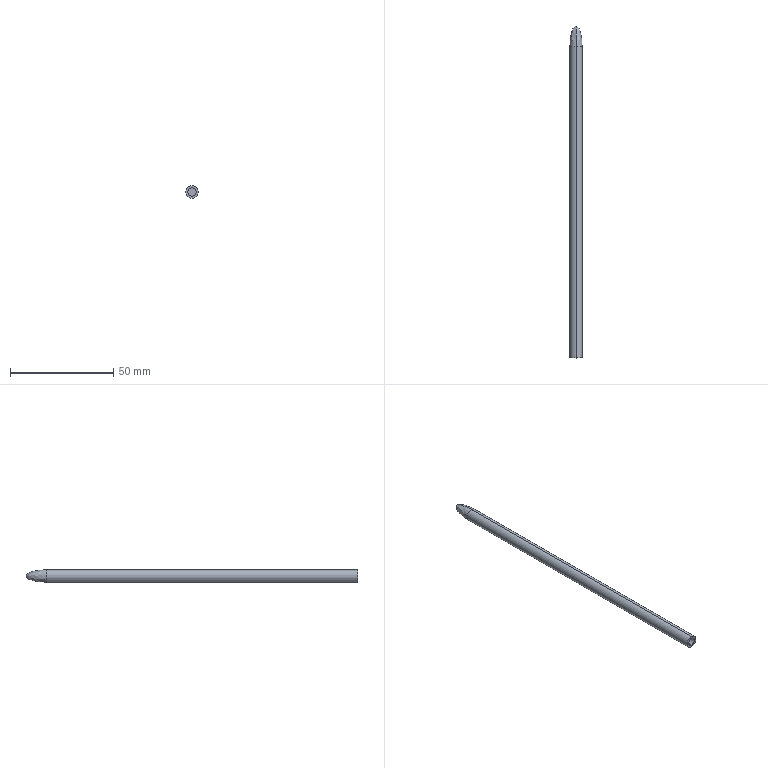Part | SolidWorks | features BaseBody 1 | 1 solid | 8 faces | box 6 x 161 x 6 mm | volume 2573 mm3 | cylinder 4 | plane 2 | spline 2 | commonest cylinder face diameters 4 x2 6 x2
STEP:
#1=CARTESIAN_POINT('',(0.,83.134,-3.));
#2=VERTEX_POINT('',#1);
#3=CARTESIAN_POINT('',(0.,83.134,3.));
#4=VERTEX_POINT('',#3);
#5=CARTESIAN_POINT('',(0.,83.134,0.));
#6=DIRECTION('',(0.,-1.,0.));
#7=DIRECTION('',(0.,0.,-1.));
#8=AXIS2_PLACEMENT_3D('',#5,#6,#7);
#9=CIRCLE('',#8,3.);
#10=EDGE_CURVE('',#2,#4,#9,.T.);
#11=ORIENTED_EDGE('',*,*,#10,.T.);
#12=CARTESIAN_POINT('',(0.,-67.866,3.));
#13=VERTEX_POINT('',#12);
#14=CARTESIAN_POINT('',(0.,0.,3.));
#15=DIRECTION('',(0.,-1.,0.));
#16=VECTOR('',#15,1000.);
#17=LINE('',#14,#16);
#18=EDGE_CURVE('',#4,#13,#17,.T.);
#19=ORIENTED_EDGE('',*,*,#18,.T.);
#20=CARTESIAN_POINT('',(0.,-67.866,-3.));
#21=VERTEX_POINT('',#20);
#22=CARTESIAN_POINT('',(0.,-67.866,0.));
#23=DIRECTION('',(0.,1.,0.));
#24=DIRECTION('',(0.,0.,-1.));
#25=AXIS2_PLACEMENT_3D('',#22,#23,#24);
#26=CIRCLE('',#25,3.);
#27=EDGE_CURVE('',#13,#21,#26,.T.);
#28=ORIENTED_EDGE('',*,*,#27,.T.);
#29=CARTESIAN_POINT('',(0.,0.,-3.));
#30=DIRECTION('',(0.,-1.,0.));
#31=VECTOR('',#30,1000.);
#32=LINE('',#29,#31);
#33=EDGE_CURVE('',#2,#21,#32,.T.);
#34=ORIENTED_EDGE('',*,*,#33,.F.);
#35=EDGE_LOOP('',(#11,#19,#28,#34));
#36=FACE_OUTER_BOUND('',#35,.T.);
#37=CARTESIAN_POINT('',(0.,0.,0.));
#38=DIRECTION('',(0.,-1.,0.));
#39=DIRECTION('',(0.,0.,-1.));
#40=AXIS2_PLACEMENT_3D('',#37,#38,#39);
#41=CYLINDRICAL_SURFACE('',#40,3.);
#42=ADVANCED_FACE('',(#36),#41,.T.);
#43=CARTESIAN_POINT('',(0.,82.134,2.));
#44=VERTEX_POINT('',#43);
#45=CARTESIAN_POINT('',(0.,82.134,-2.));
#46=VERTEX_POINT('',#45);
#47=CARTESIAN_POINT('',(0.,82.134,0.));
#48=DIRECTION('',(0.,-1.,0.));
#49=DIRECTION('',(0.,0.,-1.));
#50=AXIS2_PLACEMENT_3D('',#47,#48,#49);
#51=CIRCLE('',#50,2.);
#52=EDGE_CURVE('',#44,#46,#51,.T.);
#53=ORIENTED_EDGE('',*,*,#52,.F.);
#54=CARTESIAN_POINT('',(0.,-67.866,2.));
#55=VERTEX_POINT('',#54);
#56=CARTESIAN_POINT('',(0.,0.,2.));
#57=DIRECTION('',(0.,-1.,0.));
#58=VECTOR('',#57,1000.);
#59=LINE('',#56,#58);
#60=EDGE_CURVE('',#44,#55,#59,.T.);
#61=ORIENTED_EDGE('',*,*,#60,.T.);
#62=CARTESIAN_POINT('',(0.,-67.866,-2.));
#63=VERTEX_POINT('',#62);
#64=CARTESIAN_POINT('',(0.,-67.866,0.));
#65=DIRECTION('',(0.,-1.,0.));
#66=DIRECTION('',(0.,0.,-1.));
#67=AXIS2_PLACEMENT_3D('',#64,#65,#66);
#68=CIRCLE('',#67,2.);
#69=EDGE_CURVE('',#55,#63,#68,.T.);
#70=ORIENTED_EDGE('',*,*,#69,.T.);
#71=CARTESIAN_POINT('',(0.,0.,-2.));
#72=DIRECTION('',(0.,-1.,0.));
#73=VECTOR('',#72,1000.);
#74=LINE('',#71,#73);
#75=EDGE_CURVE('',#46,#63,#74,.T.);
#76=ORIENTED_EDGE('',*,*,#75,.F.);
#77=EDGE_LOOP('',(#53,#61,#70,#76));
#78=FACE_OUTER_BOUND('',#77,.T.);
#79=CARTESIAN_POINT('',(0.,0.,0.));
#80=DIRECTION('',(0.,-1.,0.));
#81=DIRECTION('',(0.,0.,-1.));
#82=AXIS2_PLACEMENT_3D('',#79,#80,#81);
#83=CYLINDRICAL_SURFACE('',#82,2.);
#84=ADVANCED_FACE('',(#78),#83,.F.);
#85=ORIENTED_EDGE('',*,*,#18,.F.);
#86=CARTESIAN_POINT('',(0.,83.134,0.));
#87=DIRECTION('',(0.,-1.,0.));
#88=DIRECTION('',(0.,0.,-1.));
#89=AXIS2_PLACEMENT_3D('',#86,#87,#88);
#90=CIRCLE('',#89,3.);
#91=EDGE_CURVE('',#4,#2,#90,.T.);
#92=ORIENTED_EDGE('',*,*,#91,.T.);
#93=ORIENTED_EDGE('',*,*,#33,.T.);
#94=CARTESIAN_POINT('',(0.,-67.866,0.));
#95=DIRECTION('',(0.,1.,0.));
#96=DIRECTION('',(0.,0.,-1.));
#97=AXIS2_PLACEMENT_3D('',#94,#95,#96);
#98=CIRCLE('',#97,3.);
#99=EDGE_CURVE('',#21,#13,#98,.T.);
#100=ORIENTED_EDGE('',*,*,#99,.T.);
#101=EDGE_LOOP('',(#85,#92,#93,#100));
#102=FACE_OUTER_BOUND('',#101,.T.);
#103=CARTESIAN_POINT('',(0.,0.,0.));
#104=DIRECTION('',(0.,-1.,0.));
#105=DIRECTION('',(0.,0.,-1.));
#106=AXIS2_PLACEMENT_3D('',#103,#104,#105);
#107=CYLINDRICAL_SURFACE('',#106,3.);
#108=ADVANCED_FACE('',(#102),#107,.T.);
#109=ORIENTED_EDGE('',*,*,#99,.F.);
#110=ORIENTED_EDGE('',*,*,#27,.F.);
#111=EDGE_LOOP('',(#109,#110));
#112=FACE_OUTER_BOUND('',#111,.T.);
#113=CARTESIAN_POINT('',(0.,-67.866,0.));
#114=DIRECTION('',(0.,-1.,0.));
#115=DIRECTION('',(0.,0.,-1.));
#116=AXIS2_PLACEMENT_3D('',#113,#114,#115);
#117=CIRCLE('',#116,2.);
#118=EDGE_CURVE('',#63,#55,#117,.T.);
#119=ORIENTED_EDGE('',*,*,#118,.F.);
#120=ORIENTED_EDGE('',*,*,#69,.F.);
#121=EDGE_LOOP('',(#119,#120));
#122=FACE_BOUND('',#121,.T.);
#123=CARTESIAN_POINT('',(-2.,-67.866,0.));
#124=DIRECTION('',(0.,1.,0.));
#125=DIRECTION('',(0.,0.,1.));
#126=AXIS2_PLACEMENT_3D('',#123,#124,#125);
#127=PLANE('',#126);
#128=ADVANCED_FACE('',(#112,#122),#127,.F.);
#129=CARTESIAN_POINT('',(0.,93.134,0.));
#130=VERTEX_POINT('',#129);
#131=CARTESIAN_POINT('',(0.,93.134,0.));
#132=CARTESIAN_POINT('',(0.,93.134,1.757));
#133=CARTESIAN_POINT('',(0.,88.991,3.));
#134=CARTESIAN_POINT('',(0.,83.134,3.));
#135=(BOUNDED_CURVE()B_SPLINE_CURVE(3,(#131,#132,#133,#134),.UNSPECIFIED.,.F.,.T.)B_SPLINE_CURVE_WITH_KNOTS((4,4),(0.,1.),.UNSPECIFIED.)CURVE()GEOMETRIC_REPRESENTATION_ITEM()RATIONAL_B_SPLINE_CURVE((1.,0.8047,0.8047,1.))REPRESENTATION_ITEM(''));
#136=EDGE_CURVE('',#130,#4,#135,.T.);
#137=ORIENTED_EDGE('',*,*,#136,.T.);
#138=ORIENTED_EDGE('',*,*,#10,.F.);
#139=CARTESIAN_POINT('',(0.,83.134,-3.));
#140=CARTESIAN_POINT('',(0.,88.991,-3.));
#141=CARTESIAN_POINT('',(0.,93.134,-1.757));
#142=CARTESIAN_POINT('',(0.,93.134,0.));
#143=(BOUNDED_CURVE()B_SPLINE_CURVE(3,(#139,#140,#141,#142),.UNSPECIFIED.,.F.,.F.)B_SPLINE_CURVE_WITH_KNOTS((4,4),(0.,1.),.UNSPECIFIED.)CURVE()GEOMETRIC_REPRESENTATION_ITEM()RATIONAL_B_SPLINE_CURVE((1.,0.8047,0.8047,1.))REPRESENTATION_ITEM(''));
#144=EDGE_CURVE('',#2,#130,#143,.T.);
#145=ORIENTED_EDGE('',*,*,#144,.T.);
#146=EDGE_LOOP('',(#137,#138,#145));
#147=FACE_OUTER_BOUND('',#146,.T.);
#148=CARTESIAN_POINT('',(0.,93.134,0.));
#149=CARTESIAN_POINT('',(0.,93.134,0.));
#150=CARTESIAN_POINT('',(0.,93.134,0.));
#151=CARTESIAN_POINT('',(0.,93.134,0.));
#152=CARTESIAN_POINT('',(0.,93.134,1.757));
#153=CARTESIAN_POINT('',(3.515,93.134,1.757));
#154=CARTESIAN_POINT('',(3.515,93.134,-1.757));
#155=CARTESIAN_POINT('',(0.,93.134,-1.757));
#156=CARTESIAN_POINT('',(0.,88.991,3.));
#157=CARTESIAN_POINT('',(6.,88.991,3.));
#158=CARTESIAN_POINT('',(6.,88.991,-3.));
#159=CARTESIAN_POINT('',(0.,88.991,-3.));
#160=CARTESIAN_POINT('',(0.,83.134,3.));
#161=CARTESIAN_POINT('',(6.,83.134,3.));
#162=CARTESIAN_POINT('',(6.,83.134,-3.));
#163=CARTESIAN_POINT('',(0.,83.134,-3.));
#164=(BOUNDED_SURFACE()B_SPLINE_SURFACE(3,3,((#148,#149,#150,#151),(#152,#153,#154,#155),(#156,#157,#158,#159),(#160,#161,#162,#163)),.UNSPECIFIED.,.F.,.F.,.F.)B_SPLINE_SURFACE_WITH_KNOTS((4,4),(4,4),(0.,1.),(0.,1.),.UNSPECIFIED.)GEOMETRIC_REPRESENTATION_ITEM()RATIONAL_B_SPLINE_SURFACE(((1.,0.3333,0.3333,1.),(0.8047,0.2682,0.2682,0.8047),(0.8047,0.2682,0.2682,0.8047),(1.,0.3333,0.3333,1.)))REPRESENTATION_ITEM('')SURFACE());
#165=ADVANCED_FACE('',(#147),#164,.T.);
#166=ORIENTED_EDGE('',*,*,#144,.F.);
#167=ORIENTED_EDGE('',*,*,#91,.F.);
#168=ORIENTED_EDGE('',*,*,#136,.F.);
#169=EDGE_LOOP('',(#166,#167,#168));
#170=FACE_OUTER_BOUND('',#169,.T.);
#171=CARTESIAN_POINT('',(0.,93.134,0.));
#172=CARTESIAN_POINT('',(0.,93.134,0.));
#173=CARTESIAN_POINT('',(0.,93.134,0.));
#174=CARTESIAN_POINT('',(0.,93.134,0.));
#175=CARTESIAN_POINT('',(0.,93.134,-1.757));
#176=CARTESIAN_POINT('',(-3.515,93.134,-1.757));
#177=CARTESIAN_POINT('',(-3.515,93.134,1.757));
#178=CARTESIAN_POINT('',(0.,93.134,1.757));
#179=CARTESIAN_POINT('',(0.,88.991,-3.));
#180=CARTESIAN_POINT('',(-6.,88.991,-3.));
#181=CARTESIAN_POINT('',(-6.,88.991,3.));
#182=CARTESIAN_POINT('',(0.,88.991,3.));
#183=CARTESIAN_POINT('',(0.,83.134,-3.));
#184=CARTESIAN_POINT('',(-6.,83.134,-3.));
#185=CARTESIAN_POINT('',(-6.,83.134,3.));
#186=CARTESIAN_POINT('',(0.,83.134,3.));
#187=(BOUNDED_SURFACE()B_SPLINE_SURFACE(3,3,((#171,#172,#173,#174),(#175,#176,#177,#178),(#179,#180,#181,#182),(#183,#184,#185,#186)),.UNSPECIFIED.,.F.,.F.,.F.)B_SPLINE_SURFACE_WITH_KNOTS((4,4),(4,4),(0.,1.),(0.,1.),.UNSPECIFIED.)GEOMETRIC_REPRESENTATION_ITEM()RATIONAL_B_SPLINE_SURFACE(((1.,0.3333,0.3333,1.),(0.8047,0.2682,0.2682,0.8047),(0.8047,0.2682,0.2682,0.8047),(1.,0.3333,0.3333,1.)))REPRESENTATION_ITEM('')SURFACE());
#188=ADVANCED_FACE('',(#170),#187,.T.);
#189=ORIENTED_EDGE('',*,*,#60,.F.);
#190=CARTESIAN_POINT('',(0.,82.134,0.));
#191=DIRECTION('',(0.,-1.,0.));
#192=DIRECTION('',(0.,0.,-1.));
#193=AXIS2_PLACEMENT_3D('',#190,#191,#192);
#194=CIRCLE('',#193,2.);
#195=EDGE_CURVE('',#46,#44,#194,.T.);
#196=ORIENTED_EDGE('',*,*,#195,.F.);
#197=ORIENTED_EDGE('',*,*,#75,.T.);
#198=ORIENTED_EDGE('',*,*,#118,.T.);
#199=EDGE_LOOP('',(#189,#196,#197,#198));
#200=FACE_OUTER_BOUND('',#199,.T.);
#201=CARTESIAN_POINT('',(0.,0.,0.));
#202=DIRECTION('',(0.,-1.,0.));
#203=DIRECTION('',(0.,0.,-1.));
#204=AXIS2_PLACEMENT_3D('',#201,#202,#203);
#205=CYLINDRICAL_SURFACE('',#204,2.);
#206=ADVANCED_FACE('',(#200),#205,.F.);
#207=ORIENTED_EDGE('',*,*,#195,.T.);
#208=ORIENTED_EDGE('',*,*,#52,.T.);
#209=EDGE_LOOP('',(#207,#208));
#210=FACE_OUTER_BOUND('',#209,.T.);
#211=CARTESIAN_POINT('',(0.,82.134,0.));
#212=DIRECTION('',(0.,1.,0.));
#213=DIRECTION('',(0.,0.,1.));
#214=AXIS2_PLACEMENT_3D('',#211,#212,#213);
#215=PLANE('',#214);
#216=ADVANCED_FACE('',(#210),#215,.F.);
#217=CLOSED_SHELL('',(#42,#84,#108,#128,#165,#188,#206,#216));
#218=MANIFOLD_SOLID_BREP('',#217);
#219=CARTESIAN_POINT('',(0.,0.,0.));
#220=DIRECTION('',(0.,0.,1.));
#221=DIRECTION('',(1.,0.,0.));
#222=AXIS2_PLACEMENT_3D('',#219,#220,#221);
#223=(LENGTH_UNIT()NAMED_UNIT(*)SI_UNIT(.MILLI.,.METRE.));
#224=UNCERTAINTY_MEASURE_WITH_UNIT(LENGTH_MEASURE(0.00001),#223,'','');
#225=(NAMED_UNIT(*)PLANE_ANGLE_UNIT()SI_UNIT($,.RADIAN.));
#226=(NAMED_UNIT(*)SI_UNIT($,.STERADIAN.)SOLID_ANGLE_UNIT());
#227=(GEOMETRIC_REPRESENTATION_CONTEXT(3)GLOBAL_UNCERTAINTY_ASSIGNED_CONTEXT((#224))GLOBAL_UNIT_ASSIGNED_CONTEXT((#223,#225,#226))REPRESENTATION_CONTEXT('',''));
#228=ADVANCED_BREP_SHAPE_REPRESENTATION('',(#218,#222),#227);